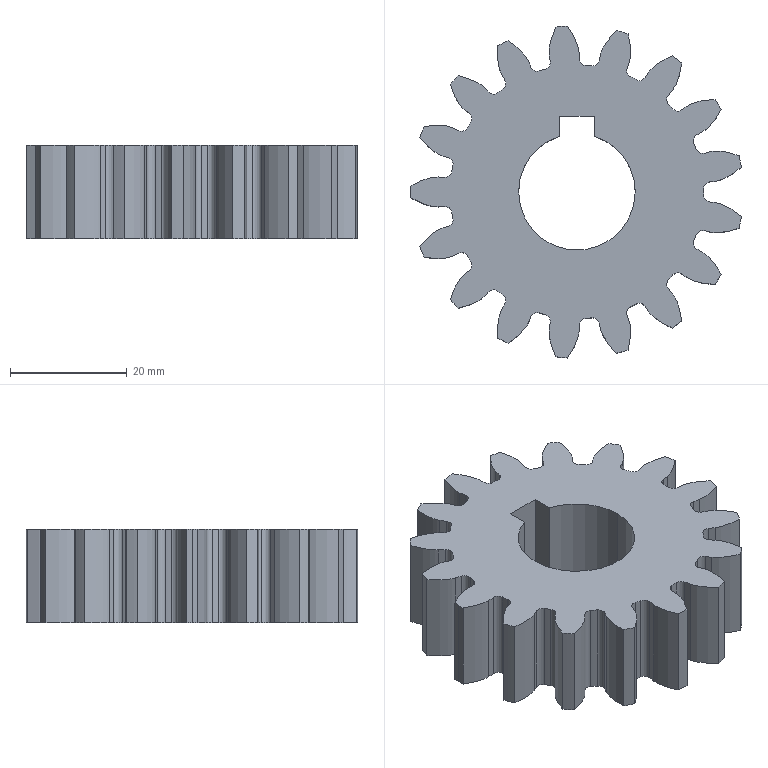Part | SolidWorks | features BaseBody 1 | 1 solid | 153 faces | box 56.683 x 56.908 x 16 mm | volume 26557 mm3 | cylinder 80 | plane 39 | spline 34 | commonest cylinder face diameters 2.28 x42 57 x18 43.5 x17 20 x3